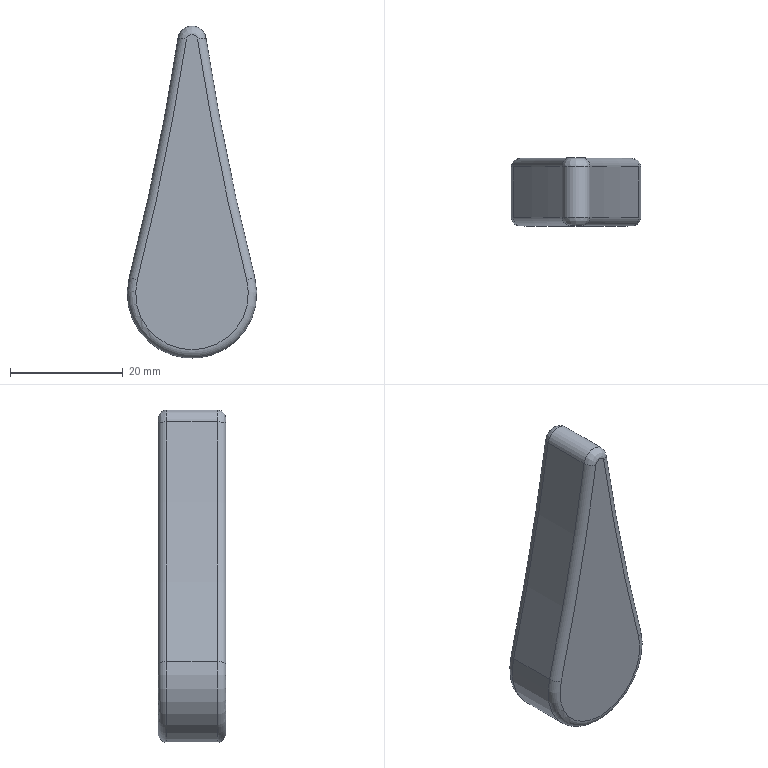Part | STEP file | CMT7E v7 | 1 solid | 14 faces | box 23 x 12 x 59 mm | volume 9832 mm3 | torus 6 | cylinder 4 | plane 2 | other 2 | commonest cylinder face diameters 930 x2 5 x1 23 x1
STEP:
#1=CARTESIAN_POINT('',(0.,0.,0.));
#2=DIRECTION('',(0.,0.,1.));
#3=DIRECTION('',(1.,0.,0.));
#4=AXIS2_PLACEMENT_3D('',#1,#2,#3);
#5=CARTESIAN_POINT('',(65.53,-55.5,227.384));
#6=VERTEX_POINT('',#5);
#7=CARTESIAN_POINT('',(70.47,-55.5,227.384));
#8=VERTEX_POINT('',#7);
#9=CARTESIAN_POINT('',(68.,-55.5,227.));
#10=DIRECTION('',(0.,1.,0.));
#11=DIRECTION('',(0.,0.,1.));
#12=AXIS2_PLACEMENT_3D('',#9,#10,#11);
#13=CIRCLE('',#12,2.5);
#14=CARTESIAN_POINT('',(68.,-54.,227.));
#15=DIRECTION('',(0.,-1.,0.));
#16=DIRECTION('',(0.9881,0.,0.1538));
#17=AXIS2_PLACEMENT_3D('',#14,#15,#16);
#18=CYLINDRICAL_SURFACE('',#17,2.5);
#19=CARTESIAN_POINT('',(7.7,1.5));
#20=DIRECTION('',(-1.,0.));
#21=VECTOR('',#20,1.);
#22=LINE('',#19,#21);
#23=(GEOMETRIC_REPRESENTATION_CONTEXT(2)PARAMETRIC_REPRESENTATION_CONTEXT()REPRESENTATION_CONTEXT('',''));
#24=DEFINITIONAL_REPRESENTATION('',(#22),#23);
#25=PCURVE('',#18,#24);
#26=CARTESIAN_POINT('',(68.,-54.,226.));
#27=CARTESIAN_POINT('',(68.,-54.,225.764));
#28=CARTESIAN_POINT('',(68.,-54.046,225.529));
#29=CARTESIAN_POINT('',(68.,-54.139,225.305));
#30=CARTESIAN_POINT('',(68.,-54.273,225.106));
#31=CARTESIAN_POINT('',(68.,-54.606,224.773));
#32=CARTESIAN_POINT('',(68.,-54.805,224.639));
#33=CARTESIAN_POINT('',(68.,-55.029,224.546));
#34=CARTESIAN_POINT('',(68.,-55.264,224.5));
#35=CARTESIAN_POINT('',(68.,-55.5,224.5));
#36=B_SPLINE_CURVE_WITH_KNOTS('',5,(#26,#27,#28,#29,#30,#31,#32,#33,#34,#35),.UNSPECIFIED.,.F.,.F.,(6,4,6),(4.712,5.498,6.283),.UNSPECIFIED.);
#37=CARTESIAN_POINT('',(68.,-55.5,227.));
#38=DIRECTION('',(0.,-1.,0.));
#39=AXIS1_PLACEMENT('',#37,#38);
#40=SURFACE_OF_REVOLUTION('',#36,#39);
#41=CARTESIAN_POINT('',(9.425,6.283));
#42=DIRECTION('',(-1.,0.));
#43=VECTOR('',#42,1.);
#44=LINE('',#41,#43);
#45=(GEOMETRIC_REPRESENTATION_CONTEXT(2)PARAMETRIC_REPRESENTATION_CONTEXT()REPRESENTATION_CONTEXT('',''));
#46=DEFINITIONAL_REPRESENTATION('',(#44),#45);
#47=PCURVE('',#40,#46);
#48=SURFACE_CURVE('',#13,(#25,#47),.PCURVE_S1.);
#49=EDGE_CURVE('',#6,#8,#48,.T.);
#50=ORIENTED_EDGE('',*,*,#49,.F.);
#51=CARTESIAN_POINT('',(65.53,-64.5,227.384));
#52=VERTEX_POINT('',#51);
#53=CARTESIAN_POINT('',(65.53,-54.,227.384));
#54=DIRECTION('',(0.,-1.,0.));
#55=VECTOR('',#54,1.);
#56=LINE('',#53,#55);
#57=CARTESIAN_POINT('',(2.833,0.));
#58=DIRECTION('',(0.,1.));
#59=VECTOR('',#58,1.);
#60=LINE('',#57,#59);
#61=(GEOMETRIC_REPRESENTATION_CONTEXT(2)PARAMETRIC_REPRESENTATION_CONTEXT()REPRESENTATION_CONTEXT('',''));
#62=DEFINITIONAL_REPRESENTATION('',(#60),#61);
#63=PCURVE('',#18,#62);
#64=CARTESIAN_POINT('',(-393.938,-54.,298.9));
#65=DIRECTION('',(0.,-1.,0.));
#66=DIRECTION('',(0.9694,0.,-0.2453));
#67=AXIS2_PLACEMENT_3D('',#64,#65,#66);
#68=CYLINDRICAL_SURFACE('',#67,465.);
#69=CARTESIAN_POINT('',(0.09345,0.));
#70=DIRECTION('',(0.,1.));
#71=VECTOR('',#70,1.);
#72=LINE('',#69,#71);
#73=(GEOMETRIC_REPRESENTATION_CONTEXT(2)PARAMETRIC_REPRESENTATION_CONTEXT()REPRESENTATION_CONTEXT('',''));
#74=DEFINITIONAL_REPRESENTATION('',(#72),#73);
#75=PCURVE('',#68,#74);
#76=SURFACE_CURVE('',#56,(#63,#75),.PCURVE_S1.);
#77=EDGE_CURVE('',#6,#52,#76,.T.);
#78=ORIENTED_EDGE('',*,*,#77,.T.);
#79=CARTESIAN_POINT('',(70.47,-64.5,227.384));
#80=VERTEX_POINT('',#79);
#81=CARTESIAN_POINT('',(68.,-64.5,227.));
#82=DIRECTION('',(0.,-1.,0.));
#83=DIRECTION('',(0.,0.,1.));
#84=AXIS2_PLACEMENT_3D('',#81,#82,#83);
#85=CIRCLE('',#84,2.5);
#86=CARTESIAN_POINT('',(-4.867,10.5));
#87=DIRECTION('',(1.,0.));
#88=VECTOR('',#87,1.);
#89=LINE('',#86,#88);
#90=(GEOMETRIC_REPRESENTATION_CONTEXT(2)PARAMETRIC_REPRESENTATION_CONTEXT()REPRESENTATION_CONTEXT('',''));
#91=DEFINITIONAL_REPRESENTATION('',(#89),#90);
#92=PCURVE('',#18,#91);
#93=CARTESIAN_POINT('',(68.,-64.5,224.5));
#94=CARTESIAN_POINT('',(68.,-64.736,224.5));
#95=CARTESIAN_POINT('',(68.,-64.971,224.546));
#96=CARTESIAN_POINT('',(68.,-65.195,224.639));
#97=CARTESIAN_POINT('',(68.,-65.394,224.773));
#98=CARTESIAN_POINT('',(68.,-65.727,225.106));
#99=CARTESIAN_POINT('',(68.,-65.861,225.305));
#100=CARTESIAN_POINT('',(68.,-65.954,225.529));
#101=CARTESIAN_POINT('',(68.,-66.,225.764));
#102=CARTESIAN_POINT('',(68.,-66.,226.));
#103=B_SPLINE_CURVE_WITH_KNOTS('',5,(#93,#94,#95,#96,#97,#98,#99,#100,#101,#102),.UNSPECIFIED.,.F.,.F.,(6,4,6),(0.,0.7854,1.571),.UNSPECIFIED.);
#104=CARTESIAN_POINT('',(68.,-64.5,227.));
#105=DIRECTION('',(0.,-1.,0.));
#106=AXIS1_PLACEMENT('',#104,#105);
#107=SURFACE_OF_REVOLUTION('',#103,#106);
#108=CARTESIAN_POINT('',(-3.142,0.));
#109=DIRECTION('',(1.,0.));
#110=VECTOR('',#109,1.);
#111=LINE('',#108,#110);
#112=(GEOMETRIC_REPRESENTATION_CONTEXT(2)PARAMETRIC_REPRESENTATION_CONTEXT()REPRESENTATION_CONTEXT('',''));
#113=DEFINITIONAL_REPRESENTATION('',(#111),#112);
#114=PCURVE('',#107,#113);
#115=SURFACE_CURVE('',#85,(#92,#114),.PCURVE_S1.);
#116=EDGE_CURVE('',#80,#52,#115,.T.);
#117=ORIENTED_EDGE('',*,*,#116,.F.);
#118=CARTESIAN_POINT('',(70.47,-54.,227.384));
#119=DIRECTION('',(0.,-1.,0.));
#120=VECTOR('',#119,1.);
#121=LINE('',#118,#120);
#122=CARTESIAN_POINT('',(0.,0.));
#123=DIRECTION('',(0.,1.));
#124=VECTOR('',#123,1.);
#125=LINE('',#122,#124);
#126=(GEOMETRIC_REPRESENTATION_CONTEXT(2)PARAMETRIC_REPRESENTATION_CONTEXT()REPRESENTATION_CONTEXT('',''));
#127=DEFINITIONAL_REPRESENTATION('',(#125),#126);
#128=PCURVE('',#18,#127);
#129=CARTESIAN_POINT('',(529.938,-54.,298.9));
#130=DIRECTION('',(0.,-1.,0.));
#131=DIRECTION('',(-0.9881,0.,-0.1538));
#132=AXIS2_PLACEMENT_3D('',#129,#130,#131);
#133=CYLINDRICAL_SURFACE('',#132,465.);
#134=CARTESIAN_POINT('',(0.,0.));
#135=DIRECTION('',(0.,1.));
#136=VECTOR('',#135,1.);
#137=LINE('',#134,#136);
#138=(GEOMETRIC_REPRESENTATION_CONTEXT(2)PARAMETRIC_REPRESENTATION_CONTEXT()REPRESENTATION_CONTEXT('',''));
#139=DEFINITIONAL_REPRESENTATION('',(#137),#138);
#140=PCURVE('',#133,#139);
#141=SURFACE_CURVE('',#121,(#128,#140),.PCURVE_S1.);
#142=EDGE_CURVE('',#8,#80,#141,.T.);
#143=ORIENTED_EDGE('',*,*,#142,.F.);
#144=EDGE_LOOP('',(#50,#78,#117,#143));
#145=FACE_BOUND('',#144,.T.);
#146=ADVANCED_FACE('',(#145),#18,.T.);
#147=CARTESIAN_POINT('',(79.149,-55.5,184.821));
#148=VERTEX_POINT('',#147);
#149=CARTESIAN_POINT('',(79.149,-64.5,184.821));
#150=VERTEX_POINT('',#149);
#151=CARTESIAN_POINT('',(79.149,-54.,184.821));
#152=DIRECTION('',(0.,-1.,0.));
#153=VECTOR('',#152,1.);
#154=LINE('',#151,#153);
#155=CARTESIAN_POINT('',(0.09345,0.));
#156=DIRECTION('',(0.,1.));
#157=VECTOR('',#156,1.);
#158=LINE('',#155,#157);
#159=(GEOMETRIC_REPRESENTATION_CONTEXT(2)PARAMETRIC_REPRESENTATION_CONTEXT()REPRESENTATION_CONTEXT('',''));
#160=DEFINITIONAL_REPRESENTATION('',(#158),#159);
#161=PCURVE('',#133,#160);
#162=CARTESIAN_POINT('',(68.,-54.,182.));
#163=DIRECTION('',(0.,-1.,0.));
#164=DIRECTION('',(0.,0.,-1.));
#165=AXIS2_PLACEMENT_3D('',#162,#163,#164);
#166=CYLINDRICAL_SURFACE('',#165,11.5);
#167=CARTESIAN_POINT('',(1.819,0.));
#168=DIRECTION('',(0.,1.));
#169=VECTOR('',#168,1.);
#170=LINE('',#167,#169);
#171=(GEOMETRIC_REPRESENTATION_CONTEXT(2)PARAMETRIC_REPRESENTATION_CONTEXT()REPRESENTATION_CONTEXT('',''));
#172=DEFINITIONAL_REPRESENTATION('',(#170),#171);
#173=PCURVE('',#166,#172);
#174=SURFACE_CURVE('',#154,(#161,#173),.PCURVE_S1.);
#175=EDGE_CURVE('',#148,#150,#174,.T.);
#176=ORIENTED_EDGE('',*,*,#175,.T.);
#177=CARTESIAN_POINT('',(529.938,-64.5,298.9));
#178=DIRECTION('',(0.,1.,0.));
#179=DIRECTION('',(-0.9798,0.,-0.1998));
#180=AXIS2_PLACEMENT_3D('',#177,#178,#179);
#181=CIRCLE('',#180,465.);
#182=CARTESIAN_POINT('',(6.33,10.5));
#183=DIRECTION('',(-1.,0.));
#184=VECTOR('',#183,1.);
#185=LINE('',#182,#184);
#186=(GEOMETRIC_REPRESENTATION_CONTEXT(2)PARAMETRIC_REPRESENTATION_CONTEXT()REPRESENTATION_CONTEXT('',''));
#187=DEFINITIONAL_REPRESENTATION('',(#185),#186);
#188=PCURVE('',#133,#187);
#189=CARTESIAN_POINT('',(529.938,-64.5,298.9));
#190=DIRECTION('',(0.,1.,0.));
#191=DIRECTION('',(0.,0.,1.));
#192=AXIS2_PLACEMENT_3D('',#189,#190,#191);
#193=TOROIDAL_SURFACE('',#192,466.5,1.5);
#194=CARTESIAN_POINT('',(-1.772,3.142));
#195=DIRECTION('',(1.,0.));
#196=VECTOR('',#195,1.);
#197=LINE('',#194,#196);
#198=(GEOMETRIC_REPRESENTATION_CONTEXT(2)PARAMETRIC_REPRESENTATION_CONTEXT()REPRESENTATION_CONTEXT('',''));
#199=DEFINITIONAL_REPRESENTATION('',(#197),#198);
#200=PCURVE('',#193,#199);
#201=SURFACE_CURVE('',#181,(#188,#200),.PCURVE_S1.);
#202=EDGE_CURVE('',#150,#80,#201,.T.);
#203=ORIENTED_EDGE('',*,*,#202,.T.);
#204=ORIENTED_EDGE('',*,*,#142,.F.);
#205=CARTESIAN_POINT('',(529.938,-55.5,298.9));
#206=DIRECTION('',(0.,-1.,0.));
#207=DIRECTION('',(-0.9798,0.,-0.1998));
#208=AXIS2_PLACEMENT_3D('',#205,#206,#207);
#209=CIRCLE('',#208,465.);
#210=CARTESIAN_POINT('',(-6.236,1.5));
#211=DIRECTION('',(1.,0.));
#212=VECTOR('',#211,1.);
#213=LINE('',#210,#212);
#214=(GEOMETRIC_REPRESENTATION_CONTEXT(2)PARAMETRIC_REPRESENTATION_CONTEXT()REPRESENTATION_CONTEXT('',''));
#215=DEFINITIONAL_REPRESENTATION('',(#213),#214);
#216=PCURVE('',#133,#215);
#217=CARTESIAN_POINT('',(529.938,-55.5,298.9));
#218=DIRECTION('',(0.,-1.,0.));
#219=DIRECTION('',(0.,0.,-1.));
#220=AXIS2_PLACEMENT_3D('',#217,#218,#219);
#221=TOROIDAL_SURFACE('',#220,466.5,1.5);
#222=CARTESIAN_POINT('',(-1.37,3.142));
#223=DIRECTION('',(1.,0.));
#224=VECTOR('',#223,1.);
#225=LINE('',#222,#224);
#226=(GEOMETRIC_REPRESENTATION_CONTEXT(2)PARAMETRIC_REPRESENTATION_CONTEXT()REPRESENTATION_CONTEXT('',''));
#227=DEFINITIONAL_REPRESENTATION('',(#225),#226);
#228=PCURVE('',#221,#227);
#229=SURFACE_CURVE('',#209,(#216,#228),.PCURVE_S1.);
#230=EDGE_CURVE('',#8,#148,#229,.T.);
#231=ORIENTED_EDGE('',*,*,#230,.T.);
#232=EDGE_LOOP('',(#176,#203,#204,#231));
#233=FACE_BOUND('',#232,.F.);
#234=ADVANCED_FACE('',(#233),#133,.F.);
#235=CARTESIAN_POINT('',(58.306,-66.,184.453));
#236=VERTEX_POINT('',#235);
#237=CARTESIAN_POINT('',(67.012,-66.,227.154));
#238=VERTEX_POINT('',#237);
#239=CARTESIAN_POINT('',(-393.938,-66.,298.9));
#240=DIRECTION('',(0.,-1.,0.));
#241=DIRECTION('',(0.9798,0.,-0.1998));
#242=AXIS2_PLACEMENT_3D('',#239,#240,#241);
#243=CIRCLE('',#242,466.5);
#244=CARTESIAN_POINT('',(68.,-66.,200.));
#245=DIRECTION('',(0.,-1.,0.));
#246=DIRECTION('',(1.,0.,0.));
#247=AXIS2_PLACEMENT_3D('',#244,#245,#246);
#248=PLANE('',#247);
#249=CARTESIAN_POINT('',(-461.938,98.9));
#250=DIRECTION('',(0.9798,-0.1998));
#251=AXIS2_PLACEMENT_2D('',#249,#250);
#252=CIRCLE('',#251,466.5);
#253=(GEOMETRIC_REPRESENTATION_CONTEXT(2)PARAMETRIC_REPRESENTATION_CONTEXT()REPRESENTATION_CONTEXT('',''));
#254=DEFINITIONAL_REPRESENTATION('',(#252),#253);
#255=PCURVE('',#248,#254);
#256=CARTESIAN_POINT('',(-393.938,-64.5,298.9));
#257=DIRECTION('',(0.,1.,0.));
#258=DIRECTION('',(0.,0.,1.));
#259=AXIS2_PLACEMENT_3D('',#256,#257,#258);
#260=TOROIDAL_SURFACE('',#259,466.5,1.5);
#261=CARTESIAN_POINT('',(8.055,4.712));
#262=DIRECTION('',(-1.,0.));
#263=VECTOR('',#262,1.);
#264=LINE('',#261,#263);
#265=(GEOMETRIC_REPRESENTATION_CONTEXT(2)PARAMETRIC_REPRESENTATION_CONTEXT()REPRESENTATION_CONTEXT('',''));
#266=DEFINITIONAL_REPRESENTATION('',(#264),#265);
#267=PCURVE('',#260,#266);
#268=SURFACE_CURVE('',#243,(#255,#267),.PCURVE_S1.);
#269=EDGE_CURVE('',#236,#238,#268,.T.);
#270=ORIENTED_EDGE('',*,*,#269,.F.);
#271=CARTESIAN_POINT('',(77.694,-66.,184.453));
#272=VERTEX_POINT('',#271);
#273=CARTESIAN_POINT('',(68.,-66.,182.));
#274=DIRECTION('',(0.,1.,0.));
#275=DIRECTION('',(0.,0.,-1.));
#276=AXIS2_PLACEMENT_3D('',#273,#274,#275);
#277=CIRCLE('',#276,10.);
#278=CARTESIAN_POINT('',(0.,-28.));
#279=CARTESIAN_POINT('',(-17.321,-28.));
#280=CARTESIAN_POINT('',(-8.66,-13.));
#281=CARTESIAN_POINT('',(0.,2.));
#282=CARTESIAN_POINT('',(8.66,-13.));
#283=CARTESIAN_POINT('',(17.321,-28.));
#284=CARTESIAN_POINT('',(0.,-28.));
#285=(BOUNDED_CURVE()B_SPLINE_CURVE(2,(#278,#279,#280,#281,#282,#283,#284),.UNSPECIFIED.,.T.,.F.)B_SPLINE_CURVE_WITH_KNOTS((1,2,2,2,2,1),(-2.094,0.,2.094,4.189,6.283,8.378),.UNSPECIFIED.)CURVE()GEOMETRIC_REPRESENTATION_ITEM()RATIONAL_B_SPLINE_CURVE((1.,0.5,1.,0.5,1.,0.5,1.))REPRESENTATION_ITEM(''));
#286=(GEOMETRIC_REPRESENTATION_CONTEXT(2)PARAMETRIC_REPRESENTATION_CONTEXT()REPRESENTATION_CONTEXT('',''));
#287=DEFINITIONAL_REPRESENTATION('',(#285),#286);
#288=PCURVE('',#248,#287);
#289=CARTESIAN_POINT('',(68.,-64.5,182.));
#290=DIRECTION('',(0.,-1.,0.));
#291=DIRECTION('',(0.,0.,-1.));
#292=AXIS2_PLACEMENT_3D('',#289,#290,#291);
#293=TOROIDAL_SURFACE('',#292,10.,1.5);
#294=CARTESIAN_POINT('',(6.283,1.571));
#295=DIRECTION('',(-1.,0.));
#296=VECTOR('',#295,1.);
#297=LINE('',#294,#296);
#298=(GEOMETRIC_REPRESENTATION_CONTEXT(2)PARAMETRIC_REPRESENTATION_CONTEXT()REPRESENTATION_CONTEXT('',''));
#299=DEFINITIONAL_REPRESENTATION('',(#297),#298);
#300=PCURVE('',#293,#299);
#301=SURFACE_CURVE('',#277,(#288,#300),.PCURVE_S1.);
#302=EDGE_CURVE('',#272,#236,#301,.T.);
#303=ORIENTED_EDGE('',*,*,#302,.F.);
#304=CARTESIAN_POINT('',(68.988,-66.,227.154));
#305=VERTEX_POINT('',#304);
#306=CARTESIAN_POINT('',(529.938,-66.,298.9));
#307=DIRECTION('',(0.,-1.,0.));
#308=DIRECTION('',(-0.9798,0.,-0.1998));
#309=AXIS2_PLACEMENT_3D('',#306,#307,#308);
#310=CIRCLE('',#309,466.5);
#311=CARTESIAN_POINT('',(461.938,98.9));
#312=DIRECTION('',(-0.9798,-0.1998));
#313=AXIS2_PLACEMENT_2D('',#311,#312);
#314=CIRCLE('',#313,466.5);
#315=(GEOMETRIC_REPRESENTATION_CONTEXT(2)PARAMETRIC_REPRESENTATION_CONTEXT()REPRESENTATION_CONTEXT('',''));
#316=DEFINITIONAL_REPRESENTATION('',(#314),#315);
#317=PCURVE('',#248,#316);
#318=CARTESIAN_POINT('',(10.794,4.712));
#319=DIRECTION('',(-1.,0.));
#320=VECTOR('',#319,1.);
#321=LINE('',#318,#320);
#322=(GEOMETRIC_REPRESENTATION_CONTEXT(2)PARAMETRIC_REPRESENTATION_CONTEXT()REPRESENTATION_CONTEXT('',''));
#323=DEFINITIONAL_REPRESENTATION('',(#321),#322);
#324=PCURVE('',#193,#323);
#325=SURFACE_CURVE('',#310,(#317,#324),.PCURVE_S1.);
#326=EDGE_CURVE('',#305,#272,#325,.T.);
#327=ORIENTED_EDGE('',*,*,#326,.F.);
#328=CARTESIAN_POINT('',(68.,-66.,227.));
#329=DIRECTION('',(0.,1.,0.));
#330=DIRECTION('',(0.,0.,1.));
#331=AXIS2_PLACEMENT_3D('',#328,#329,#330);
#332=CIRCLE('',#331,1.);
#333=CARTESIAN_POINT('',(0.,28.));
#334=CARTESIAN_POINT('',(1.732,28.));
#335=CARTESIAN_POINT('',(0.866,26.5));
#336=CARTESIAN_POINT('',(0.,25.));
#337=CARTESIAN_POINT('',(-0.866,26.5));
#338=CARTESIAN_POINT('',(-1.732,28.));
#339=CARTESIAN_POINT('',(0.,28.));
#340=(BOUNDED_CURVE()B_SPLINE_CURVE(2,(#333,#334,#335,#336,#337,#338,#339),.UNSPECIFIED.,.T.,.F.)B_SPLINE_CURVE_WITH_KNOTS((1,2,2,2,2,1),(-2.094,0.,2.094,4.189,6.283,8.378),.UNSPECIFIED.)CURVE()GEOMETRIC_REPRESENTATION_ITEM()RATIONAL_B_SPLINE_CURVE((1.,0.5,1.,0.5,1.,0.5,1.))REPRESENTATION_ITEM(''));
#341=(GEOMETRIC_REPRESENTATION_CONTEXT(2)PARAMETRIC_REPRESENTATION_CONTEXT()REPRESENTATION_CONTEXT('',''));
#342=DEFINITIONAL_REPRESENTATION('',(#340),#341);
#343=PCURVE('',#248,#342);
#344=CARTESIAN_POINT('',(9.425,1.571));
#345=DIRECTION('',(-1.,0.));
#346=VECTOR('',#345,1.);
#347=LINE('',#344,#346);
#348=(GEOMETRIC_REPRESENTATION_CONTEXT(2)PARAMETRIC_REPRESENTATION_CONTEXT()REPRESENTATION_CONTEXT('',''));
#349=DEFINITIONAL_REPRESENTATION('',(#347),#348);
#350=PCURVE('',#107,#349);
#351=SURFACE_CURVE('',#332,(#343,#350),.PCURVE_S1.);
#352=EDGE_CURVE('',#238,#305,#351,.T.);
#353=ORIENTED_EDGE('',*,*,#352,.F.);
#354=EDGE_LOOP('',(#270,#303,#327,#353));
#355=FACE_BOUND('',#354,.T.);
#356=ADVANCED_FACE('',(#355),#248,.T.);
#357=CARTESIAN_POINT('',(67.012,-64.5,227.154));
#358=DIRECTION('',(-0.1538,0.,-0.9881));
#359=DIRECTION('',(0.,-1.,0.));
#360=AXIS2_PLACEMENT_3D('',#357,#358,#359);
#361=CIRCLE('',#360,1.5);
#362=CARTESIAN_POINT('',(4.558,1.571));
#363=CARTESIAN_POINT('',(4.558,1.547));
#364=CARTESIAN_POINT('',(4.558,1.499));
#365=CARTESIAN_POINT('',(4.558,1.428));
#366=CARTESIAN_POINT('',(4.558,1.357));
#367=CARTESIAN_POINT('',(4.558,1.285));
#368=CARTESIAN_POINT('',(4.558,1.214));
#369=CARTESIAN_POINT('',(4.558,1.142));
#370=CARTESIAN_POINT('',(4.558,1.071));
#371=CARTESIAN_POINT('',(4.558,0.9996));
#372=CARTESIAN_POINT('',(4.558,0.9282));
#373=CARTESIAN_POINT('',(4.558,0.8568));
#374=CARTESIAN_POINT('',(4.558,0.7854));
#375=CARTESIAN_POINT('',(4.558,0.714));
#376=CARTESIAN_POINT('',(4.558,0.6426));
#377=CARTESIAN_POINT('',(4.558,0.5712));
#378=CARTESIAN_POINT('',(4.558,0.4998));
#379=CARTESIAN_POINT('',(4.558,0.4284));
#380=CARTESIAN_POINT('',(4.558,0.357));
#381=CARTESIAN_POINT('',(4.558,0.2856));
#382=CARTESIAN_POINT('',(4.558,0.2142));
#383=CARTESIAN_POINT('',(4.558,0.1428));
#384=CARTESIAN_POINT('',(4.558,0.0714));
#385=CARTESIAN_POINT('',(4.558,0.0238));
#386=CARTESIAN_POINT('',(4.558,0.));
#387=B_SPLINE_CURVE_WITH_KNOTS('',3,(#362,#363,#364,#365,#366,#367,#368,#369,#370,#371,#372,#373,#374,#375,#376,#377,#378,#379,#380,#381,#382,#383,#384,#385,#386),.UNSPECIFIED.,.F.,.F.,(4,1,1,1,1,1,1,1,1,1,1,1,1,1,1,1,1,1,1,1,1,1,4),(0.,0.0714,0.1428,0.2142,0.2856,0.357,0.4284,0.4998,0.5712,0.6426,0.714,0.7854,0.8568,0.9282,0.9996,1.071,1.142,1.214,1.285,1.357,1.428,1.499,1.571),.QUASI_UNIFORM_KNOTS.);
#388=(GEOMETRIC_REPRESENTATION_CONTEXT(2)PARAMETRIC_REPRESENTATION_CONTEXT()REPRESENTATION_CONTEXT('',''));
#389=DEFINITIONAL_REPRESENTATION('',(#387),#388);
#390=PCURVE('',#107,#389);
#391=CARTESIAN_POINT('',(1.725,4.712));
#392=DIRECTION('',(0.,-1.));
#393=VECTOR('',#392,1.);
#394=LINE('',#391,#393);
#395=(GEOMETRIC_REPRESENTATION_CONTEXT(2)PARAMETRIC_REPRESENTATION_CONTEXT()REPRESENTATION_CONTEXT('',''));
#396=DEFINITIONAL_REPRESENTATION('',(#394),#395);
#397=PCURVE('',#260,#396);
#398=SURFACE_CURVE('',#361,(#390,#397),.PCURVE_S1.);
#399=EDGE_CURVE('',#238,#52,#398,.T.);
#400=ORIENTED_EDGE('',*,*,#399,.F.);
#401=ORIENTED_EDGE('',*,*,#352,.T.);
#402=CARTESIAN_POINT('',(68.988,-64.5,227.154));
#403=DIRECTION('',(0.1538,0.,-0.9881));
#404=DIRECTION('',(0.9881,0.,0.1538));
#405=AXIS2_PLACEMENT_3D('',#402,#403,#404);
#406=CIRCLE('',#405,1.5);
#407=CARTESIAN_POINT('',(1.725,0.));
#408=CARTESIAN_POINT('',(1.725,0.0238));
#409=CARTESIAN_POINT('',(1.725,0.0714));
#410=CARTESIAN_POINT('',(1.725,0.1428));
#411=CARTESIAN_POINT('',(1.725,0.2142));
#412=CARTESIAN_POINT('',(1.725,0.2856));
#413=CARTESIAN_POINT('',(1.725,0.357));
#414=CARTESIAN_POINT('',(1.725,0.4284));
#415=CARTESIAN_POINT('',(1.725,0.4998));
#416=CARTESIAN_POINT('',(1.725,0.5712));
#417=CARTESIAN_POINT('',(1.725,0.6426));
#418=CARTESIAN_POINT('',(1.725,0.714));
#419=CARTESIAN_POINT('',(1.725,0.7854));
#420=CARTESIAN_POINT('',(1.725,0.8568));
#421=CARTESIAN_POINT('',(1.725,0.9282));
#422=CARTESIAN_POINT('',(1.725,0.9996));
#423=CARTESIAN_POINT('',(1.725,1.071));
#424=CARTESIAN_POINT('',(1.725,1.142));
#425=CARTESIAN_POINT('',(1.725,1.214));
#426=CARTESIAN_POINT('',(1.725,1.285));
#427=CARTESIAN_POINT('',(1.725,1.357));
#428=CARTESIAN_POINT('',(1.725,1.428));
#429=CARTESIAN_POINT('',(1.725,1.499));
#430=CARTESIAN_POINT('',(1.725,1.547));
#431=CARTESIAN_POINT('',(1.725,1.571));
#432=B_SPLINE_CURVE_WITH_KNOTS('',3,(#407,#408,#409,#410,#411,#412,#413,#414,#415,#416,#417,#418,#419,#420,#421,#422,#423,#424,#425,#426,#427,#428,#429,#430,#431),.UNSPECIFIED.,.F.,.F.,(4,1,1,1,1,1,1,1,1,1,1,1,1,1,1,1,1,1,1,1,1,1,4),(0.,0.0714,0.1428,0.2142,0.2856,0.357,0.4284,0.4998,0.5712,0.6426,0.714,0.7854,0.8568,0.9282,0.9996,1.071,1.142,1.214,1.285,1.357,1.428,1.499,1.571),.QUASI_UNIFORM_KNOTS.);
#433=(GEOMETRIC_REPRESENTATION_CONTEXT(2)PARAMETRIC_REPRESENTATION_CONTEXT()REPRESENTATION_CONTEXT('',''));
#434=DEFINITIONAL_REPRESENTATION('',(#432),#433);
#435=PCURVE('',#107,#434);
#436=CARTESIAN_POINT('',(4.558,3.142));
#437=DIRECTION('',(0.,1.));
#438=VECTOR('',#437,1.);
#439=LINE('',#436,#438);
#440=(GEOMETRIC_REPRESENTATION_CONTEXT(2)PARAMETRIC_REPRESENTATION_CONTEXT()REPRESENTATION_CONTEXT('',''));
#441=DEFINITIONAL_REPRESENTATION('',(#439),#440);
#442=PCURVE('',#193,#441);
#443=SURFACE_CURVE('',#406,(#435,#442),.PCURVE_S1.);
#444=EDGE_CURVE('',#80,#305,#443,.T.);
#445=ORIENTED_EDGE('',*,*,#444,.F.);
#446=ORIENTED_EDGE('',*,*,#116,.T.);
#447=EDGE_LOOP('',(#400,#401,#445,#446));
#448=FACE_BOUND('',#447,.T.);
#449=ADVANCED_FACE('',(#448),#107,.T.);
#450=ORIENTED_EDGE('',*,*,#444,.T.);
#451=ORIENTED_EDGE('',*,*,#326,.T.);
#452=CARTESIAN_POINT('',(77.694,-64.5,184.453));
#453=DIRECTION('',(0.2453,0.,-0.9694));
#454=DIRECTION('',(0.9694,0.,0.2453));
#455=AXIS2_PLACEMENT_3D('',#452,#453,#454);
#456=CIRCLE('',#455,1.5);
#457=CARTESIAN_POINT('',(4.465,3.142));
#458=DIRECTION('',(0.,1.));
#459=VECTOR('',#458,1.);
#460=LINE('',#457,#459);
#461=(GEOMETRIC_REPRESENTATION_CONTEXT(2)PARAMETRIC_REPRESENTATION_CONTEXT()REPRESENTATION_CONTEXT('',''));
#462=DEFINITIONAL_REPRESENTATION('',(#460),#461);
#463=PCURVE('',#193,#462);
#464=CARTESIAN_POINT('',(1.819,0.));
#465=DIRECTION('',(0.,1.));
#466=VECTOR('',#465,1.);
#467=LINE('',#464,#466);
#468=(GEOMETRIC_REPRESENTATION_CONTEXT(2)PARAMETRIC_REPRESENTATION_CONTEXT()REPRESENTATION_CONTEXT('',''));
#469=DEFINITIONAL_REPRESENTATION('',(#467),#468);
#470=PCURVE('',#293,#469);
#471=SURFACE_CURVE('',#456,(#463,#470),.PCURVE_S1.);
#472=EDGE_CURVE('',#150,#272,#471,.T.);
#473=ORIENTED_EDGE('',*,*,#472,.F.);
#474=ORIENTED_EDGE('',*,*,#202,.T.);
#475=EDGE_LOOP('',(#450,#451,#473,#474));
#476=FACE_BOUND('',#475,.T.);
#477=ADVANCED_FACE('',(#476),#193,.T.);
#478=ORIENTED_EDGE('',*,*,#472,.T.);
#479=ORIENTED_EDGE('',*,*,#302,.T.);
#480=CARTESIAN_POINT('',(56.851,-64.5,184.821));
#481=VERTEX_POINT('',#480);
#482=CARTESIAN_POINT('',(58.306,-64.5,184.453));
#483=DIRECTION('',(0.2453,0.,0.9694));
#484=DIRECTION('',(-0.9694,0.,0.2453));
#485=AXIS2_PLACEMENT_3D('',#482,#483,#484);
#486=CIRCLE('',#485,1.5);
#487=CARTESIAN_POINT('',(-1.819,0.));
#488=DIRECTION('',(0.,1.));
#489=VECTOR('',#488,1.);
#490=LINE('',#487,#489);
#491=(GEOMETRIC_REPRESENTATION_CONTEXT(2)PARAMETRIC_REPRESENTATION_CONTEXT()REPRESENTATION_CONTEXT('',''));
#492=DEFINITIONAL_REPRESENTATION('',(#490),#491);
#493=PCURVE('',#293,#492);
#494=CARTESIAN_POINT('',(1.819,3.142));
#495=DIRECTION('',(0.,1.));
#496=VECTOR('',#495,1.);
#497=LINE('',#494,#496);
#498=(GEOMETRIC_REPRESENTATION_CONTEXT(2)PARAMETRIC_REPRESENTATION_CONTEXT()REPRESENTATION_CONTEXT('',''));
#499=DEFINITIONAL_REPRESENTATION('',(#497),#498);
#500=PCURVE('',#260,#499);
#501=SURFACE_CURVE('',#486,(#493,#500),.PCURVE_S1.);
#502=EDGE_CURVE('',#481,#236,#501,.T.);
#503=ORIENTED_EDGE('',*,*,#502,.F.);
#504=CARTESIAN_POINT('',(68.,-64.5,182.));
#505=DIRECTION('',(0.,-1.,0.));
#506=DIRECTION('',(0.,0.,-1.));
#507=AXIS2_PLACEMENT_3D('',#504,#505,#506);
#508=CIRCLE('',#507,11.5);
#509=CARTESIAN_POINT('',(-6.283,0.));
#510=DIRECTION('',(1.,0.));
#511=VECTOR('',#510,1.);
#512=LINE('',#509,#511);
#513=(GEOMETRIC_REPRESENTATION_CONTEXT(2)PARAMETRIC_REPRESENTATION_CONTEXT()REPRESENTATION_CONTEXT('',''));
#514=DEFINITIONAL_REPRESENTATION('',(#512),#513);
#515=PCURVE('',#293,#514);
#516=CARTESIAN_POINT('',(-6.283,10.5));
#517=DIRECTION('',(1.,0.));
#518=VECTOR('',#517,1.);
#519=LINE('',#516,#518);
#520=(GEOMETRIC_REPRESENTATION_CONTEXT(2)PARAMETRIC_REPRESENTATION_CONTEXT()REPRESENTATION_CONTEXT('',''));
#521=DEFINITIONAL_REPRESENTATION('',(#519),#520);
#522=PCURVE('',#166,#521);
#523=SURFACE_CURVE('',#508,(#515,#522),.PCURVE_S1.);
#524=EDGE_CURVE('',#481,#150,#523,.T.);
#525=ORIENTED_EDGE('',*,*,#524,.T.);
#526=EDGE_LOOP('',(#478,#479,#503,#525));
#527=FACE_BOUND('',#526,.T.);
#528=ADVANCED_FACE('',(#527),#293,.T.);
#529=ORIENTED_EDGE('',*,*,#399,.T.);
#530=CARTESIAN_POINT('',(-393.938,-64.5,298.9));
#531=DIRECTION('',(0.,1.,0.));
#532=DIRECTION('',(0.9798,0.,-0.1998));
#533=AXIS2_PLACEMENT_3D('',#530,#531,#532);
#534=CIRCLE('',#533,465.);
#535=CARTESIAN_POINT('',(-4.511,3.142));
#536=DIRECTION('',(1.,0.));
#537=VECTOR('',#536,1.);
#538=LINE('',#535,#537);
#539=(GEOMETRIC_REPRESENTATION_CONTEXT(2)PARAMETRIC_REPRESENTATION_CONTEXT()REPRESENTATION_CONTEXT('',''));
#540=DEFINITIONAL_REPRESENTATION('',(#538),#539);
#541=PCURVE('',#260,#540);
#542=CARTESIAN_POINT('',(6.33,10.5));
#543=DIRECTION('',(-1.,0.));
#544=VECTOR('',#543,1.);
#545=LINE('',#542,#544);
#546=(GEOMETRIC_REPRESENTATION_CONTEXT(2)PARAMETRIC_REPRESENTATION_CONTEXT()REPRESENTATION_CONTEXT('',''));
#547=DEFINITIONAL_REPRESENTATION('',(#545),#546);
#548=PCURVE('',#68,#547);
#549=SURFACE_CURVE('',#534,(#541,#548),.PCURVE_S1.);
#550=EDGE_CURVE('',#52,#481,#549,.T.);
#551=ORIENTED_EDGE('',*,*,#550,.T.);
#552=ORIENTED_EDGE('',*,*,#502,.T.);
#553=ORIENTED_EDGE('',*,*,#269,.T.);
#554=EDGE_LOOP('',(#529,#551,#552,#553));
#555=FACE_BOUND('',#554,.T.);
#556=ADVANCED_FACE('',(#555),#260,.T.);
#557=CARTESIAN_POINT('',(58.306,-54.,184.453));
#558=VERTEX_POINT('',#557);
#559=CARTESIAN_POINT('',(77.694,-54.,184.453));
#560=VERTEX_POINT('',#559);
#561=CARTESIAN_POINT('',(68.,-54.,182.));
#562=DIRECTION('',(0.,-1.,0.));
#563=DIRECTION('',(0.,0.,-1.));
#564=AXIS2_PLACEMENT_3D('',#561,#562,#563);
#565=CIRCLE('',#564,10.);
#566=CARTESIAN_POINT('',(68.,-54.,200.));
#567=DIRECTION('',(0.,-1.,0.));
#568=DIRECTION('',(1.,0.,0.));
#569=AXIS2_PLACEMENT_3D('',#566,#567,#568);
#570=PLANE('',#569);
#571=CARTESIAN_POINT('',(0.,-18.));
#572=DIRECTION('',(0.,-1.));
#573=AXIS2_PLACEMENT_2D('',#571,#572);
#574=CIRCLE('',#573,10.);
#575=(GEOMETRIC_REPRESENTATION_CONTEXT(2)PARAMETRIC_REPRESENTATION_CONTEXT()REPRESENTATION_CONTEXT('',''));
#576=DEFINITIONAL_REPRESENTATION('',(#574),#575);
#577=PCURVE('',#570,#576);
#578=CARTESIAN_POINT('',(68.,-55.5,182.));
#579=DIRECTION('',(0.,-1.,0.));
#580=DIRECTION('',(0.,0.,-1.));
#581=AXIS2_PLACEMENT_3D('',#578,#579,#580);
#582=TOROIDAL_SURFACE('',#581,10.,1.5);
#583=CARTESIAN_POINT('',(-6.283,4.712));
#584=DIRECTION('',(1.,0.));
#585=VECTOR('',#584,1.);
#586=LINE('',#583,#585);
#587=(GEOMETRIC_REPRESENTATION_CONTEXT(2)PARAMETRIC_REPRESENTATION_CONTEXT()REPRESENTATION_CONTEXT('',''));
#588=DEFINITIONAL_REPRESENTATION('',(#586),#587);
#589=PCURVE('',#582,#588);
#590=SURFACE_CURVE('',#565,(#577,#589),.PCURVE_S1.);
#591=EDGE_CURVE('',#558,#560,#590,.T.);
#592=ORIENTED_EDGE('',*,*,#591,.F.);
#593=CARTESIAN_POINT('',(67.012,-54.,227.154));
#594=VERTEX_POINT('',#593);
#595=CARTESIAN_POINT('',(-393.938,-54.,298.9));
#596=DIRECTION('',(0.,1.,0.));
#597=DIRECTION('',(0.9798,0.,-0.1998));
#598=AXIS2_PLACEMENT_3D('',#595,#596,#597);
#599=CIRCLE('',#598,466.5);
#600=CARTESIAN_POINT('',(-4.842,5.702));
#601=CARTESIAN_POINT('',(-166.266,-786.011));
#602=CARTESIAN_POINT('',(-771.198,-250.357));
#603=CARTESIAN_POINT('',(-1376.129,285.296));
#604=CARTESIAN_POINT('',(-609.774,541.355));
#605=CARTESIAN_POINT('',(156.582,797.415));
#606=CARTESIAN_POINT('',(-4.842,5.702));
#607=(BOUNDED_CURVE()B_SPLINE_CURVE(2,(#600,#601,#602,#603,#604,#605,#606),.UNSPECIFIED.,.T.,.F.)B_SPLINE_CURVE_WITH_KNOTS((1,2,2,2,2,1),(-2.094,0.,2.094,4.189,6.283,8.378),.UNSPECIFIED.)CURVE()GEOMETRIC_REPRESENTATION_ITEM()RATIONAL_B_SPLINE_CURVE((1.,0.5,1.,0.5,1.,0.5,1.))REPRESENTATION_ITEM(''));
#608=(GEOMETRIC_REPRESENTATION_CONTEXT(2)PARAMETRIC_REPRESENTATION_CONTEXT()REPRESENTATION_CONTEXT('',''));
#609=DEFINITIONAL_REPRESENTATION('',(#607),#608);
#610=PCURVE('',#570,#609);
#611=CARTESIAN_POINT('',(-393.938,-55.5,298.9));
#612=DIRECTION('',(0.,-1.,0.));
#613=DIRECTION('',(0.,0.,-1.));
#614=AXIS2_PLACEMENT_3D('',#611,#612,#613);
#615=TOROIDAL_SURFACE('',#614,466.5,1.5);
#616=CARTESIAN_POINT('',(7.653,4.712));
#617=DIRECTION('',(-1.,0.));
#618=VECTOR('',#617,1.);
#619=LINE('',#616,#618);
#620=(GEOMETRIC_REPRESENTATION_CONTEXT(2)PARAMETRIC_REPRESENTATION_CONTEXT()REPRESENTATION_CONTEXT('',''));
#621=DEFINITIONAL_REPRESENTATION('',(#619),#620);
#622=PCURVE('',#615,#621);
#623=SURFACE_CURVE('',#599,(#610,#622),.PCURVE_S1.);
#624=EDGE_CURVE('',#594,#558,#623,.T.);
#625=ORIENTED_EDGE('',*,*,#624,.F.);
#626=CARTESIAN_POINT('',(68.988,-54.,227.154));
#627=VERTEX_POINT('',#626);
#628=CARTESIAN_POINT('',(68.,-54.,227.));
#629=DIRECTION('',(0.,-1.,0.));
#630=DIRECTION('',(0.,0.,1.));
#631=AXIS2_PLACEMENT_3D('',#628,#629,#630);
#632=CIRCLE('',#631,1.);
#633=CARTESIAN_POINT('',(0.,27.));
#634=DIRECTION('',(0.,1.));
#635=AXIS2_PLACEMENT_2D('',#633,#634);
#636=CIRCLE('',#635,1.);
#637=(GEOMETRIC_REPRESENTATION_CONTEXT(2)PARAMETRIC_REPRESENTATION_CONTEXT()REPRESENTATION_CONTEXT('',''));
#638=DEFINITIONAL_REPRESENTATION('',(#636),#637);
#639=PCURVE('',#570,#638);
#640=CARTESIAN_POINT('',(-3.142,4.712));
#641=DIRECTION('',(1.,0.));
#642=VECTOR('',#641,1.);
#643=LINE('',#640,#642);
#644=(GEOMETRIC_REPRESENTATION_CONTEXT(2)PARAMETRIC_REPRESENTATION_CONTEXT()REPRESENTATION_CONTEXT('',''));
#645=DEFINITIONAL_REPRESENTATION('',(#643),#644);
#646=PCURVE('',#40,#645);
#647=SURFACE_CURVE('',#632,(#639,#646),.PCURVE_S1.);
#648=EDGE_CURVE('',#627,#594,#647,.T.);
#649=ORIENTED_EDGE('',*,*,#648,.F.);
#650=CARTESIAN_POINT('',(529.938,-54.,298.9));
#651=DIRECTION('',(0.,1.,0.));
#652=DIRECTION('',(-0.9798,0.,-0.1998));
#653=AXIS2_PLACEMENT_3D('',#650,#651,#652);
#654=CIRCLE('',#653,466.5);
#655=CARTESIAN_POINT('',(4.842,5.702));
#656=CARTESIAN_POINT('',(-156.582,797.415));
#657=CARTESIAN_POINT('',(609.774,541.355));
#658=CARTESIAN_POINT('',(1376.129,285.296));
#659=CARTESIAN_POINT('',(771.198,-250.357));
#660=CARTESIAN_POINT('',(166.266,-786.011));
#661=CARTESIAN_POINT('',(4.842,5.702));
#662=(BOUNDED_CURVE()B_SPLINE_CURVE(2,(#655,#656,#657,#658,#659,#660,#661),.UNSPECIFIED.,.T.,.F.)B_SPLINE_CURVE_WITH_KNOTS((1,2,2,2,2,1),(-2.094,0.,2.094,4.189,6.283,8.378),.UNSPECIFIED.)CURVE()GEOMETRIC_REPRESENTATION_ITEM()RATIONAL_B_SPLINE_CURVE((1.,0.5,1.,0.5,1.,0.5,1.))REPRESENTATION_ITEM(''));
#663=(GEOMETRIC_REPRESENTATION_CONTEXT(2)PARAMETRIC_REPRESENTATION_CONTEXT()REPRESENTATION_CONTEXT('',''));
#664=DEFINITIONAL_REPRESENTATION('',(#662),#663);
#665=PCURVE('',#570,#664);
#666=CARTESIAN_POINT('',(11.197,4.712));
#667=DIRECTION('',(-1.,0.));
#668=VECTOR('',#667,1.);
#669=LINE('',#666,#668);
#670=(GEOMETRIC_REPRESENTATION_CONTEXT(2)PARAMETRIC_REPRESENTATION_CONTEXT()REPRESENTATION_CONTEXT('',''));
#671=DEFINITIONAL_REPRESENTATION('',(#669),#670);
#672=PCURVE('',#221,#671);
#673=SURFACE_CURVE('',#654,(#665,#672),.PCURVE_S1.);
#674=EDGE_CURVE('',#560,#627,#673,.T.);
#675=ORIENTED_EDGE('',*,*,#674,.F.);
#676=EDGE_LOOP('',(#592,#625,#649,#675));
#677=FACE_BOUND('',#676,.T.);
#678=ADVANCED_FACE('',(#677),#570,.F.);
#679=CARTESIAN_POINT('',(56.851,-55.5,184.821));
#680=VERTEX_POINT('',#679);
#681=CARTESIAN_POINT('',(68.,-55.5,182.));
#682=DIRECTION('',(0.,1.,0.));
#683=DIRECTION('',(0.,0.,-1.));
#684=AXIS2_PLACEMENT_3D('',#681,#682,#683);
#685=CIRCLE('',#684,11.5);
#686=CARTESIAN_POINT('',(6.283,1.5));
#687=DIRECTION('',(-1.,0.));
#688=VECTOR('',#687,1.);
#689=LINE('',#686,#688);
#690=(GEOMETRIC_REPRESENTATION_CONTEXT(2)PARAMETRIC_REPRESENTATION_CONTEXT()REPRESENTATION_CONTEXT('',''));
#691=DEFINITIONAL_REPRESENTATION('',(#689),#690);
#692=PCURVE('',#166,#691);
#693=CARTESIAN_POINT('',(6.283,6.283));
#694=DIRECTION('',(-1.,0.));
#695=VECTOR('',#694,1.);
#696=LINE('',#693,#695);
#697=(GEOMETRIC_REPRESENTATION_CONTEXT(2)PARAMETRIC_REPRESENTATION_CONTEXT()REPRESENTATION_CONTEXT('',''));
#698=DEFINITIONAL_REPRESENTATION('',(#696),#697);
#699=PCURVE('',#582,#698);
#700=SURFACE_CURVE('',#685,(#692,#699),.PCURVE_S1.);
#701=EDGE_CURVE('',#148,#680,#700,.T.);
#702=ORIENTED_EDGE('',*,*,#701,.F.);
#703=ORIENTED_EDGE('',*,*,#175,.T.);
#704=ORIENTED_EDGE('',*,*,#524,.F.);
#705=CARTESIAN_POINT('',(56.851,-54.,184.821));
#706=DIRECTION('',(0.,-1.,0.));
#707=VECTOR('',#706,1.);
#708=LINE('',#705,#707);
#709=CARTESIAN_POINT('',(-1.819,0.));
#710=DIRECTION('',(0.,1.));
#711=VECTOR('',#710,1.);
#712=LINE('',#709,#711);
#713=(GEOMETRIC_REPRESENTATION_CONTEXT(2)PARAMETRIC_REPRESENTATION_CONTEXT()REPRESENTATION_CONTEXT('',''));
#714=DEFINITIONAL_REPRESENTATION('',(#712),#713);
#715=PCURVE('',#166,#714);
#716=CARTESIAN_POINT('',(0.,0.));
#717=DIRECTION('',(0.,1.));
#718=VECTOR('',#717,1.);
#719=LINE('',#716,#718);
#720=(GEOMETRIC_REPRESENTATION_CONTEXT(2)PARAMETRIC_REPRESENTATION_CONTEXT()REPRESENTATION_CONTEXT('',''));
#721=DEFINITIONAL_REPRESENTATION('',(#719),#720);
#722=PCURVE('',#68,#721);
#723=SURFACE_CURVE('',#708,(#715,#722),.PCURVE_S1.);
#724=EDGE_CURVE('',#680,#481,#723,.T.);
#725=ORIENTED_EDGE('',*,*,#724,.F.);
#726=EDGE_LOOP('',(#702,#703,#704,#725));
#727=FACE_BOUND('',#726,.T.);
#728=ADVANCED_FACE('',(#727),#166,.T.);
#729=ORIENTED_EDGE('',*,*,#77,.T.);
#730=ORIENTED_EDGE('',*,*,#550,.T.);
#731=ORIENTED_EDGE('',*,*,#724,.F.);
#732=CARTESIAN_POINT('',(-393.938,-55.5,298.9));
#733=DIRECTION('',(0.,-1.,0.));
#734=DIRECTION('',(0.9798,0.,-0.1998));
#735=AXIS2_PLACEMENT_3D('',#732,#733,#734);
#736=CIRCLE('',#735,465.);
#737=CARTESIAN_POINT('',(-6.236,1.5));
#738=DIRECTION('',(1.,0.));
#739=VECTOR('',#738,1.);
#740=LINE('',#737,#739);
#741=(GEOMETRIC_REPRESENTATION_CONTEXT(2)PARAMETRIC_REPRESENTATION_CONTEXT()REPRESENTATION_CONTEXT('',''));
#742=DEFINITIONAL_REPRESENTATION('',(#740),#741);
#743=PCURVE('',#68,#742);
#744=CARTESIAN_POINT('',(-4.914,3.142));
#745=DIRECTION('',(1.,0.));
#746=VECTOR('',#745,1.);
#747=LINE('',#744,#746);
#748=(GEOMETRIC_REPRESENTATION_CONTEXT(2)PARAMETRIC_REPRESENTATION_CONTEXT()REPRESENTATION_CONTEXT('',''));
#749=DEFINITIONAL_REPRESENTATION('',(#747),#748);
#750=PCURVE('',#615,#749);
#751=SURFACE_CURVE('',#736,(#743,#750),.PCURVE_S1.);
#752=EDGE_CURVE('',#680,#6,#751,.T.);
#753=ORIENTED_EDGE('',*,*,#752,.T.);
#754=EDGE_LOOP('',(#729,#730,#731,#753));
#755=FACE_BOUND('',#754,.F.);
#756=ADVANCED_FACE('',(#755),#68,.F.);
#757=CARTESIAN_POINT('',(67.012,-55.5,227.154));
#758=DIRECTION('',(0.1538,0.,0.9881));
#759=DIRECTION('',(0.,1.,0.));
#760=AXIS2_PLACEMENT_3D('',#757,#758,#759);
#761=CIRCLE('',#760,1.5);
#762=CARTESIAN_POINT('',(1.416,4.712));
#763=DIRECTION('',(0.,-1.));
#764=VECTOR('',#763,1.);
#765=LINE('',#762,#764);
#766=(GEOMETRIC_REPRESENTATION_CONTEXT(2)PARAMETRIC_REPRESENTATION_CONTEXT()REPRESENTATION_CONTEXT('',''));
#767=DEFINITIONAL_REPRESENTATION('',(#765),#766);
#768=PCURVE('',#615,#767);
#769=CARTESIAN_POINT('',(4.558,4.712));
#770=CARTESIAN_POINT('',(4.558,4.736));
#771=CARTESIAN_POINT('',(4.558,4.784));
#772=CARTESIAN_POINT('',(4.558,4.855));
#773=CARTESIAN_POINT('',(4.558,4.927));
#774=CARTESIAN_POINT('',(4.558,4.998));
#775=CARTESIAN_POINT('',(4.558,5.069));
#776=CARTESIAN_POINT('',(4.558,5.141));
#777=CARTESIAN_POINT('',(4.558,5.212));
#778=CARTESIAN_POINT('',(4.558,5.284));
#779=CARTESIAN_POINT('',(4.558,5.355));
#780=CARTESIAN_POINT('',(4.558,5.426));
#781=CARTESIAN_POINT('',(4.558,5.498));
#782=CARTESIAN_POINT('',(4.558,5.569));
#783=CARTESIAN_POINT('',(4.558,5.641));
#784=CARTESIAN_POINT('',(4.558,5.712));
#785=CARTESIAN_POINT('',(4.558,5.783));
#786=CARTESIAN_POINT('',(4.558,5.855));
#787=CARTESIAN_POINT('',(4.558,5.926));
#788=CARTESIAN_POINT('',(4.558,5.998));
#789=CARTESIAN_POINT('',(4.558,6.069));
#790=CARTESIAN_POINT('',(4.558,6.14));
#791=CARTESIAN_POINT('',(4.558,6.212));
#792=CARTESIAN_POINT('',(4.558,6.259));
#793=CARTESIAN_POINT('',(4.558,6.283));
#794=B_SPLINE_CURVE_WITH_KNOTS('',3,(#769,#770,#771,#772,#773,#774,#775,#776,#777,#778,#779,#780,#781,#782,#783,#784,#785,#786,#787,#788,#789,#790,#791,#792,#793),.UNSPECIFIED.,.F.,.F.,(4,1,1,1,1,1,1,1,1,1,1,1,1,1,1,1,1,1,1,1,1,1,4),(0.,0.0714,0.1428,0.2142,0.2856,0.357,0.4284,0.4998,0.5712,0.6426,0.714,0.7854,0.8568,0.9282,0.9996,1.071,1.142,1.214,1.285,1.357,1.428,1.499,1.571),.QUASI_UNIFORM_KNOTS.);
#795=(GEOMETRIC_REPRESENTATION_CONTEXT(2)PARAMETRIC_REPRESENTATION_CONTEXT()REPRESENTATION_CONTEXT('',''));
#796=DEFINITIONAL_REPRESENTATION('',(#794),#795);
#797=PCURVE('',#40,#796);
#798=SURFACE_CURVE('',#761,(#768,#797),.PCURVE_S1.);
#799=EDGE_CURVE('',#594,#6,#798,.T.);
#800=ORIENTED_EDGE('',*,*,#799,.F.);
#801=ORIENTED_EDGE('',*,*,#624,.T.);
#802=CARTESIAN_POINT('',(58.306,-55.5,184.453));
#803=DIRECTION('',(-0.2453,0.,-0.9694));
#804=DIRECTION('',(-0.9694,0.,0.2453));
#805=AXIS2_PLACEMENT_3D('',#802,#803,#804);
#806=CIRCLE('',#805,1.5);
#807=CARTESIAN_POINT('',(1.323,3.142));
#808=DIRECTION('',(0.,1.));
#809=VECTOR('',#808,1.);
#810=LINE('',#807,#809);
#811=(GEOMETRIC_REPRESENTATION_CONTEXT(2)PARAMETRIC_REPRESENTATION_CONTEXT()REPRESENTATION_CONTEXT('',''));
#812=DEFINITIONAL_REPRESENTATION('',(#810),#811);
#813=PCURVE('',#615,#812);
#814=CARTESIAN_POINT('',(-1.819,6.283));
#815=DIRECTION('',(0.,-1.));
#816=VECTOR('',#815,1.);
#817=LINE('',#814,#816);
#818=(GEOMETRIC_REPRESENTATION_CONTEXT(2)PARAMETRIC_REPRESENTATION_CONTEXT()REPRESENTATION_CONTEXT('',''));
#819=DEFINITIONAL_REPRESENTATION('',(#817),#818);
#820=PCURVE('',#582,#819);
#821=SURFACE_CURVE('',#806,(#813,#820),.PCURVE_S1.);
#822=EDGE_CURVE('',#680,#558,#821,.T.);
#823=ORIENTED_EDGE('',*,*,#822,.F.);
#824=ORIENTED_EDGE('',*,*,#752,.T.);
#825=EDGE_LOOP('',(#800,#801,#823,#824));
#826=FACE_BOUND('',#825,.T.);
#827=ADVANCED_FACE('',(#826),#615,.T.);
#828=ORIENTED_EDGE('',*,*,#799,.T.);
#829=ORIENTED_EDGE('',*,*,#49,.T.);
#830=CARTESIAN_POINT('',(68.988,-55.5,227.154));
#831=DIRECTION('',(0.1538,0.,-0.9881));
#832=DIRECTION('',(0.,1.,0.));
#833=AXIS2_PLACEMENT_3D('',#830,#831,#832);
#834=CIRCLE('',#833,1.5);
#835=CARTESIAN_POINT('',(1.725,4.712));
#836=CARTESIAN_POINT('',(1.725,4.736));
#837=CARTESIAN_POINT('',(1.725,4.784));
#838=CARTESIAN_POINT('',(1.725,4.855));
#839=CARTESIAN_POINT('',(1.725,4.927));
#840=CARTESIAN_POINT('',(1.725,4.998));
#841=CARTESIAN_POINT('',(1.725,5.069));
#842=CARTESIAN_POINT('',(1.725,5.141));
#843=CARTESIAN_POINT('',(1.725,5.212));
#844=CARTESIAN_POINT('',(1.725,5.284));
#845=CARTESIAN_POINT('',(1.725,5.355));
#846=CARTESIAN_POINT('',(1.725,5.426));
#847=CARTESIAN_POINT('',(1.725,5.498));
#848=CARTESIAN_POINT('',(1.725,5.569));
#849=CARTESIAN_POINT('',(1.725,5.641));
#850=CARTESIAN_POINT('',(1.725,5.712));
#851=CARTESIAN_POINT('',(1.725,5.783));
#852=CARTESIAN_POINT('',(1.725,5.855));
#853=CARTESIAN_POINT('',(1.725,5.926));
#854=CARTESIAN_POINT('',(1.725,5.998));
#855=CARTESIAN_POINT('',(1.725,6.069));
#856=CARTESIAN_POINT('',(1.725,6.14));
#857=CARTESIAN_POINT('',(1.725,6.212));
#858=CARTESIAN_POINT('',(1.725,6.259));
#859=CARTESIAN_POINT('',(1.725,6.283));
#860=B_SPLINE_CURVE_WITH_KNOTS('',3,(#835,#836,#837,#838,#839,#840,#841,#842,#843,#844,#845,#846,#847,#848,#849,#850,#851,#852,#853,#854,#855,#856,#857,#858,#859),.UNSPECIFIED.,.F.,.F.,(4,1,1,1,1,1,1,1,1,1,1,1,1,1,1,1,1,1,1,1,1,1,4),(0.,0.0714,0.1428,0.2142,0.2856,0.357,0.4284,0.4998,0.5712,0.6426,0.714,0.7854,0.8568,0.9282,0.9996,1.071,1.142,1.214,1.285,1.357,1.428,1.499,1.571),.QUASI_UNIFORM_KNOTS.);
#861=(GEOMETRIC_REPRESENTATION_CONTEXT(2)PARAMETRIC_REPRESENTATION_CONTEXT()REPRESENTATION_CONTEXT('',''));
#862=DEFINITIONAL_REPRESENTATION('',(#860),#861);
#863=PCURVE('',#40,#862);
#864=CARTESIAN_POINT('',(4.867,4.712));
#865=DIRECTION('',(0.,-1.));
#866=VECTOR('',#865,1.);
#867=LINE('',#864,#866);
#868=(GEOMETRIC_REPRESENTATION_CONTEXT(2)PARAMETRIC_REPRESENTATION_CONTEXT()REPRESENTATION_CONTEXT('',''));
#869=DEFINITIONAL_REPRESENTATION('',(#867),#868);
#870=PCURVE('',#221,#869);
#871=SURFACE_CURVE('',#834,(#863,#870),.PCURVE_S1.);
#872=EDGE_CURVE('',#627,#8,#871,.T.);
#873=ORIENTED_EDGE('',*,*,#872,.F.);
#874=ORIENTED_EDGE('',*,*,#648,.T.);
#875=EDGE_LOOP('',(#828,#829,#873,#874));
#876=FACE_BOUND('',#875,.T.);
#877=ADVANCED_FACE('',(#876),#40,.T.);
#878=ORIENTED_EDGE('',*,*,#872,.T.);
#879=ORIENTED_EDGE('',*,*,#230,.T.);
#880=CARTESIAN_POINT('',(77.694,-55.5,184.453));
#881=DIRECTION('',(0.2453,0.,-0.9694));
#882=DIRECTION('',(0.,1.,0.));
#883=AXIS2_PLACEMENT_3D('',#880,#881,#882);
#884=CIRCLE('',#883,1.5);
#885=CARTESIAN_POINT('',(4.96,4.712));
#886=DIRECTION('',(0.,-1.));
#887=VECTOR('',#886,1.);
#888=LINE('',#885,#887);
#889=(GEOMETRIC_REPRESENTATION_CONTEXT(2)PARAMETRIC_REPRESENTATION_CONTEXT()REPRESENTATION_CONTEXT('',''));
#890=DEFINITIONAL_REPRESENTATION('',(#888),#889);
#891=PCURVE('',#221,#890);
#892=CARTESIAN_POINT('',(1.819,4.712));
#893=DIRECTION('',(0.,1.));
#894=VECTOR('',#893,1.);
#895=LINE('',#892,#894);
#896=(GEOMETRIC_REPRESENTATION_CONTEXT(2)PARAMETRIC_REPRESENTATION_CONTEXT()REPRESENTATION_CONTEXT('',''));
#897=DEFINITIONAL_REPRESENTATION('',(#895),#896);
#898=PCURVE('',#582,#897);
#899=SURFACE_CURVE('',#884,(#891,#898),.PCURVE_S1.);
#900=EDGE_CURVE('',#560,#148,#899,.T.);
#901=ORIENTED_EDGE('',*,*,#900,.F.);
#902=ORIENTED_EDGE('',*,*,#674,.T.);
#903=EDGE_LOOP('',(#878,#879,#901,#902));
#904=FACE_BOUND('',#903,.T.);
#905=ADVANCED_FACE('',(#904),#221,.T.);
#906=ORIENTED_EDGE('',*,*,#822,.T.);
#907=ORIENTED_EDGE('',*,*,#591,.T.);
#908=ORIENTED_EDGE('',*,*,#900,.T.);
#909=ORIENTED_EDGE('',*,*,#701,.T.);
#910=EDGE_LOOP('',(#906,#907,#908,#909));
#911=FACE_BOUND('',#910,.T.);
#912=ADVANCED_FACE('',(#911),#582,.T.);
#913=CLOSED_SHELL('',(#146,#234,#356,#449,#477,#528,#556,#678,#728,#756,#827,#877,#905,#912));
#914=MANIFOLD_SOLID_BREP('',#913);
#915=(LENGTH_UNIT()NAMED_UNIT(*)SI_UNIT(.MILLI.,.METRE.));
#916=UNCERTAINTY_MEASURE_WITH_UNIT(LENGTH_MEASURE(0.0000005),#915,'','');
#917=(NAMED_UNIT(*)PLANE_ANGLE_UNIT()SI_UNIT($,.RADIAN.));
#918=(NAMED_UNIT(*)SI_UNIT($,.STERADIAN.)SOLID_ANGLE_UNIT());
#919=(GEOMETRIC_REPRESENTATION_CONTEXT(3)GLOBAL_UNCERTAINTY_ASSIGNED_CONTEXT((#916))GLOBAL_UNIT_ASSIGNED_CONTEXT((#915,#917,#918))REPRESENTATION_CONTEXT('',''));
#920=ADVANCED_BREP_SHAPE_REPRESENTATION('',(#4,#914),#919);